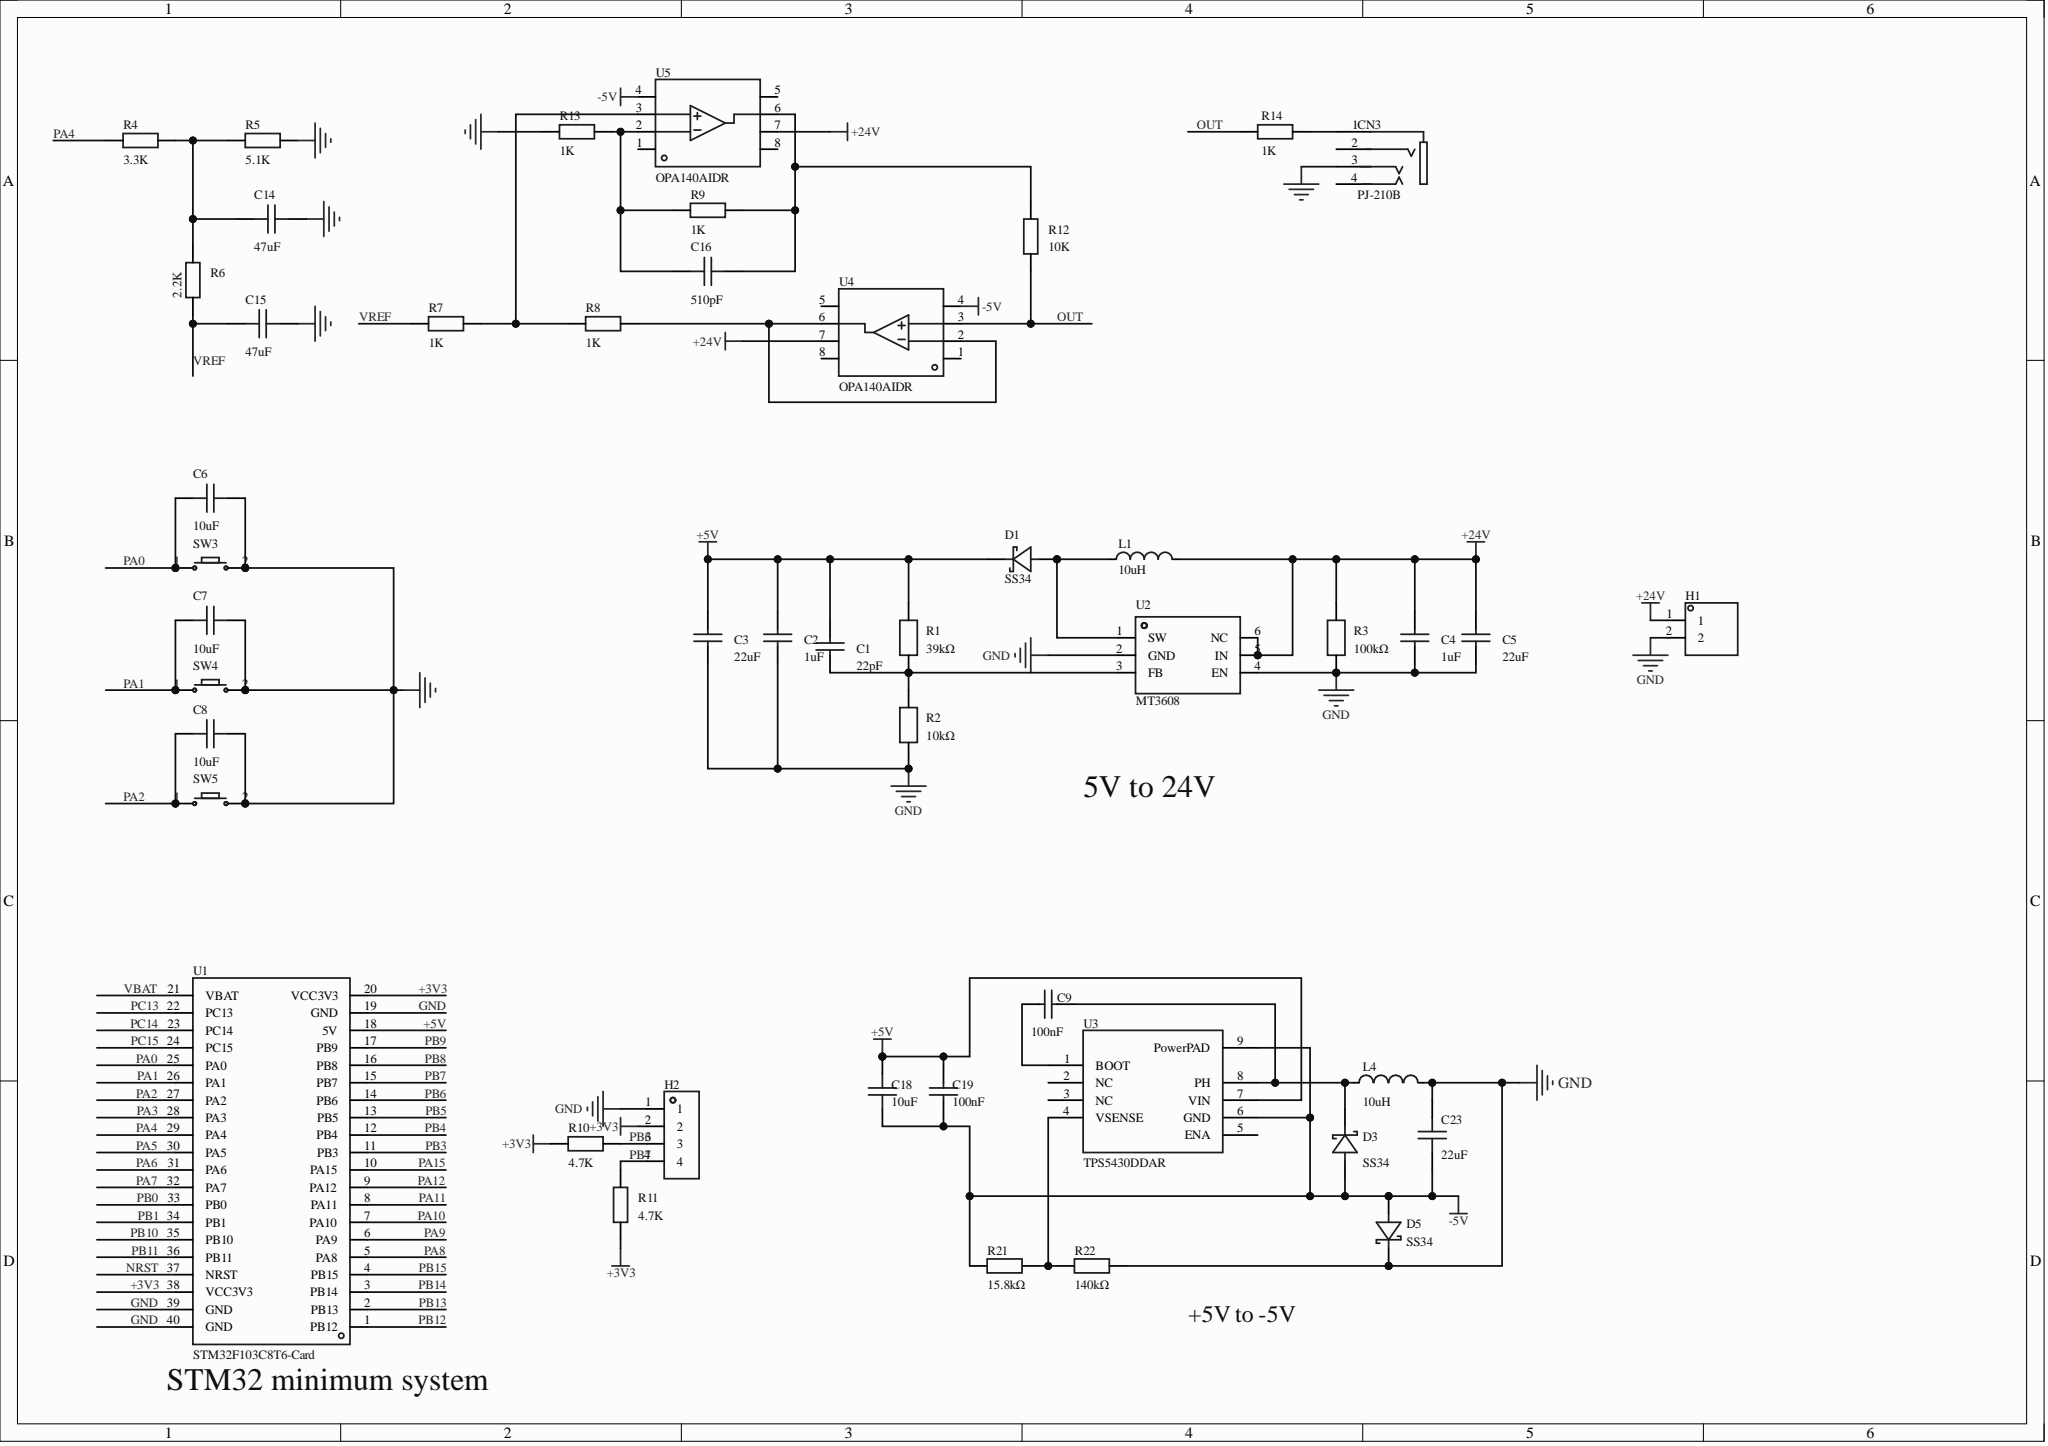Circuit board | Altium Designer | 47 parts | 24 nets
Bill of materials:
Comment,Description,Designator,Footprint,LibRef,Quantity
"22pF","Capacitance: 22pF; Tolerance: ±5%; Rated voltage: 50V; Temperature coefficient: NP0;","C1","C0603","CC0603JRNPO9BN220","1"
"1uF","Capacitance: 22pF; Tolerance: ±5%; Rated voltage: 50V; Temperature coefficient: NP0;","C2, C4","C0603","CC0603JRNPO9BN220","2"
"22uF","Capacitance: 22pF; Tolerance: ±5%; Rated voltage: 50V; Temperature coefficient: NP0;","C3, C5","C0603","CC0603JRNPO9BN220","2"
"10uF","","C6, C7, C8","C0603","CAP_0603","3"
"100nF","Capacitance: 100nF; Tolerance: ±10%; Rated voltage: 25V; Dielectric (temperature coefficient): X7R;","C9","C0603","CL10B104KA8NNNC","1"
"47uF","","C14, C15","C0603","CAP_0603","2"
"510pF","","C16","C0603","CAP_0603","1"
"10uF","Capacitance: 10uF; Tolerance: ±10%; Rated voltage: 50V; Temperature coefficient: X5R;","C18","C1206","HGC1206R5106K500NSPJ","1"
"100nF","Capacitance: 100nF; Tolerance: ±10%; Rated voltage: 100V; Dielectric (temperature coefficient): X7R;","C19","C0805","CL21B104KCFNNNE","1"
"22uF","Capacitance: 22uF; Tolerance: ±20%; Rated voltage: 25V; Dielectric (temperature coefficient): X5R;","C23","C0805","CL21A226MAQNNNE","1"
"PJ-210B","Connector type: 2.5mm earphone jack; Rated current: 500mA; Rated voltage: 30V; Operating temperature: -30℃~+70℃;","CN3","AUDIO-TH_PJ-210B","PJ-210B","1"
"SS34","Diode configuration: single; Forward voltage (Vf): 550mV@3A; DC reverse voltage (Vr): 40V; Rectified current: 3A;, Diode configuration: single; Forward voltage (Vf): 550mV@3.0A; DC reverse voltage (Vr): 40V; Average rectified current (Io): 3A;","D1, D3, D5","SMA_L4.3-W2.6-LS5.0-FD","SS34_C7420365","3"
"","","H1","HDR-TH_2P-P2.54-V-M-1","HDR-M_2.54_1x2P","1"
"","","H2","HDR-TH_4P-P2.54-V-F","HDR-F_2.54_1x4P","1"
"10uH","Inductance: 10uH; Tolerance: ±20%; Rated current: 3.2A; Saturation current (Isat): 3.5A; Type: molded inductor;","L1","IND-SMD_L6.0-W5.2_SUMIDA_CDH53","PCR0530-100-M","1"
"10uH","Inductance: 15uH; Tolerance: ±20%; Rated current: 3A; Saturation current (Isat): 4A; Type: -;","L4","IND-SMD_L7.3-W6.8","MWSA0603S-150MT","1"
"39kΩ","Resistor type: thick film resistor; Resistance: 160kΩ; Tolerance: ±1%; Power: 100mW; Operating voltage: 75V; Temperature coefficient: ±100ppm/?;","R1","R0603","FRC0603F1603TS","1"
"10kΩ","Resistor type: thick film resistor; Resistance: 160kΩ; Tolerance: ±1%; Power: 100mW; Operating voltage: 75V; Temperature coefficient: ±100ppm/?;","R2","R0603","FRC0603F1603TS","1"
"100kΩ","Resistor type: thick film resistor; Resistance: 160kΩ; Tolerance: ±1%; Power: 100mW; Operating voltage: 75V; Temperature coefficient: ±100ppm/?;","R3","R0603","FRC0603F1603TS","1"
"3.3K","","R4","R0603","Res_0603","1"
"5.1K","","R5","R0603","Res_0603","1"
"2.2K","","R6","R0603","Res_0603","1"
"1K","","R7, R8, R9, R13, R14","R0603","Res_0603","5"
"4.7K","","R10, R11","R0603","Res_0603","2"
"10K","","R12","R0603","Res_0603","1"
"15.8kΩ","Resistor type: thick film resistor; Resistance: 15.8kΩ; Tolerance: ±1%; Power: 100mW; Max operating voltage: 75V; Temperature coefficient: ±100ppm/?;","R21","R0603","0603WAF1582T5E","1"
"140kΩ","Resistor type: thick film resistor; Resistance: 140kΩ; Tolerance: ±1%; Power: 100mW; Max operating voltage: 75V; Temperature coefficient: ±100ppm/?;","R22","R0603","0603WAF1403T5E","1"
"","","SW3, SW4, SW5","Key_SMD_3x4x2","Key_SMD_3x4x2","3"
"STM32F103C8T6-Card","","U1","CONN-TH_L53.3-W22.9_STM32F103C8T6-CARD","STM32F103C8T6-Card","1"
"MT3608","Function type: boost; Output type: adjustable; Operating voltage: 2V~24V; Output voltage: -; Output current: 2A;","U2","SOT-23-6_L2.9-W1.6-P0.95-LS2.8-BL","MT3608","1"
"TPS5430DDAR","Function type: buck; Output type: adjustable; Operating voltage: 5.5V~36V; Output voltage: 1.221V~32.04V; Output current: 3A;","U3","ESOP-8_L4.9-W3.9-P1.27-LS6.0-TL-EP","TPS5430DDAR","1"
"OPA140AIDR","Amplifier count: single; Gain-bandwidth product (GBP): 11MHz; Slew rate (SR): 20V/us;","U4, U5","SOIC-8_L5.0-W4.0-P1.27-LS6.0-BL","OPA140AIDR","2"
Netlist (Protel format):
[
C1
C0603
22pF



]
[
C2
C0603
1uF



]
[
C3
C0603
22uF



]
[
C4
C0603
1uF



]
[
C5
C0603
22uF



]
[
C6
C0603
10uF



]
[
C7
C0603
10uF



]
[
C8
C0603
10uF



]
[
C9
C0603
100nF



]
[
C14
C0603
47uF



]
[
C15
C0603
47uF



]
[
C16
C0603
510pF



]
[
C18
C1206
10uF



]
[
C19
C0805
100nF



]
[
C23
C0805
22uF



]
[
CN3
AUDIO-TH_PJ-210B
PJ-210B



]
[
D1
SMA_L4.3-W2.6-LS5.0-FD
SS34



]
[
D3
SMA_L4.3-W2.6-LS5.0-FD
SS34



]
[
D5
SMA_L4.3-W2.6-LS5.0-FD
SS34



]
[
H1
HDR-TH_2P-P2.54-V-M-1




]
[
H2
HDR-TH_4P-P2.54-V-F




]
[
L1
IND-SMD_L6.0-W5.2_SUMIDA_CDH53
10uH



]
[
L4
IND-SMD_L7.3-W6.8
10uH



]
[
R1
R0603
39kΩ



]
[
R2
R0603
10kΩ



]
[
R3
R0603
100kΩ



]
[
R4
R0603
3.3K



]
[
R5
R0603
5.1K



]
[
R6
R0603
2.2K



]
[
R7
R0603
1K



]
[
R8
R0603
1K



]
[
R9
R0603
1K



]
[
R10
R0603
4.7K



]
[
R11
R0603
4.7K



]
[
R12
R0603
10K



]
[
R13
R0603
1K



]
[
R14
R0603
1K



]
[
R21
R0603
15.8kΩ



]
[
R22
R0603
140kΩ



]
[
SW3
Key_SMD_3x4x2




]
[
SW4
Key_SMD_3x4x2




]
[
SW5
Key_SMD_3x4x2




]
[
U1
CONN-TH_L53.3-W22.9_STM32F103C8T6-CARD
STM32F103C8T6-Card



]
[
U2
SOT-23-6_L2.9-W1.6-P0.95-LS2.8-BL
MT3608



]
[
U3
ESOP-8_L4.9-W3.9-P1.27-LS6.0-TL-EP
TPS5430DDAR



]
[
U4
SOIC-8_L5.0-W4.0-P1.27-LS6.0-BL
OPA140AIDR



]
[
U5
SOIC-8_L5.0-W4.0-P1.27-LS6.0-BL
OPA140AIDR



]
(
VREF
C15-1
R6-1
R7-1
)
(
PB7
H2-4
R11-2
U1-15
)
(
PB6
H2-3
R10-2
U1-14
)
(
PA4
R4-1
U1-29
)
(
PA2
C8-1
SW5-1
U1-27
)
(
PA1
C7-1
SW4-1
U1-26
)
(
PA0
C6-1
SW3-1
U1-25
)
(
OUT
R12-1
R14-2
U4-3
)
(
NetR21_2
R21-2
R22-1
U3-4
)
(
NetR8_2
R8-2
U4-2
U4-6
)
(
NetR7_2
R7-2
R8-1
U5-3
)
(
NetD1_1
D1-1
L1-1
U2-1
)
(
NetCN3_1
CN3-1
R14-1
)
(
NetC16_2
C16-2
R9-2
R12-2
U5-6
)
(
NetC16_1
C16-1
R9-1
R13-2
U5-2
)
(
NetC14_1
C14-1
R4-2
R5-1
R6-2
)
(
NetC9_2
C9-2
D3-2
L4-1
U3-8
)
(
NetC9_1
C9-1
U3-1
)
(
NetC1_1
C1-1
R1-1
R2-2
U2-3
)
(
GND
C2-1
C3-1
C4-1
C5-1
C6-2
C7-2
C8-2
C14-2
C15-2
C23-2
CN3-3
D5-2
H1-2
H2-1
L4-2
R2-1
R3-1
R5-2
R13-1
R22-2
SW3-2
SW4-2
SW5-2
U1-19
U1-39
U1-40
U2-2
U2-4
)
(
-5V
C18-1
C19-1
C23-1
D3-1
D5-1
R21-1
U3-6
U3-9
U4-4
U5-4
)
(
+24V
C4-2
C5-2
H1-1
L1-2
R3-2
U2-5
U2-6
U4-7
U5-7
)
(
+5V
C1-2
C2-2
C3-2
C18-2
C19-2
D1-2
R1-2
U1-18
U3-7
)
(
+3V3
H2-2
R10-1
R11-1
U1-20
U1-38
)